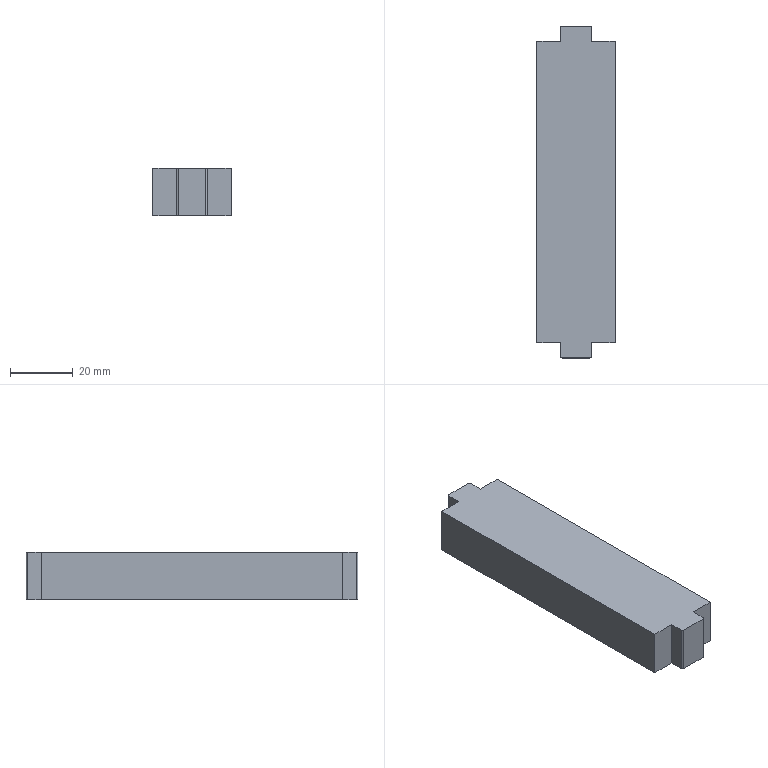Part | STEP file | 1 solid | 27 faces | box 25 x 105.8 x 15 mm | volume 36908 mm3 | plane 14 | cylinder 7 | cone 6 | commonest cylinder face diameters 0.9 x4 4.2 x3